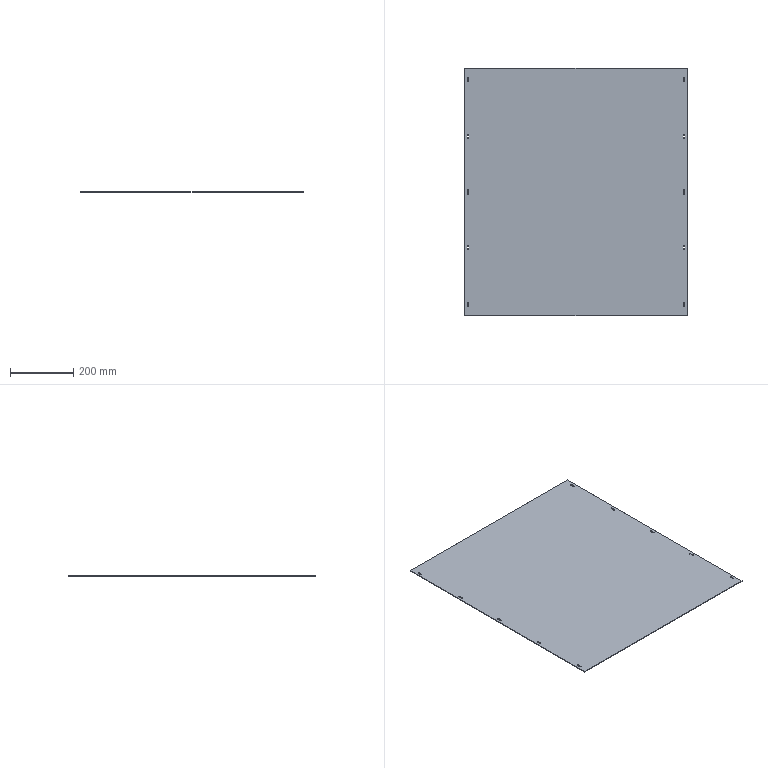Part | SolidWorks | features Extrusion 1, ICE 1 | 1 solid | 46 faces | box 700 x 780 x 2 mm | volume 1090782 mm3 | plane 26 | cylinder 20 | commonest cylinder face diameters 4.5 x20
STEP:
#1=CARTESIAN_POINT('',(350.,-390.,0.));
#2=VERTEX_POINT('',#1);
#3=CARTESIAN_POINT('',(350.,390.,0.));
#4=VERTEX_POINT('',#3);
#5=CARTESIAN_POINT('',(350.,390.,0.));
#6=DIRECTION('',(0.,1.,0.));
#7=VECTOR('',#6,1000.);
#8=LINE('',#5,#7);
#9=EDGE_CURVE('',#2,#4,#8,.T.);
#10=ORIENTED_EDGE('',*,*,#9,.T.);
#11=CARTESIAN_POINT('',(350.,390.,2.));
#12=VERTEX_POINT('',#11);
#13=CARTESIAN_POINT('',(350.,390.,2.));
#14=DIRECTION('',(0.,0.,-1.));
#15=VECTOR('',#14,1000.);
#16=LINE('',#13,#15);
#17=EDGE_CURVE('',#12,#4,#16,.T.);
#18=ORIENTED_EDGE('',*,*,#17,.F.);
#19=CARTESIAN_POINT('',(350.,-390.,2.));
#20=VERTEX_POINT('',#19);
#21=CARTESIAN_POINT('',(350.,390.,2.));
#22=DIRECTION('',(0.,1.,0.));
#23=VECTOR('',#22,1000.);
#24=LINE('',#21,#23);
#25=EDGE_CURVE('',#20,#12,#24,.T.);
#26=ORIENTED_EDGE('',*,*,#25,.F.);
#27=CARTESIAN_POINT('',(350.,-390.,2.));
#28=DIRECTION('',(0.,0.,-1.));
#29=VECTOR('',#28,1000.);
#30=LINE('',#27,#29);
#31=EDGE_CURVE('',#20,#2,#30,.T.);
#32=ORIENTED_EDGE('',*,*,#31,.T.);
#33=EDGE_LOOP('',(#10,#18,#26,#32));
#34=FACE_OUTER_BOUND('',#33,.T.);
#35=CARTESIAN_POINT('',(350.,390.,2.));
#36=DIRECTION('',(-1.,0.,0.));
#37=DIRECTION('',(0.,0.,1.));
#38=AXIS2_PLACEMENT_3D('',#35,#36,#37);
#39=PLANE('',#38);
#40=ADVANCED_FACE('',(#34),#39,.F.);
#41=CARTESIAN_POINT('',(-350.,390.,0.));
#42=VERTEX_POINT('',#41);
#43=CARTESIAN_POINT('',(-350.,390.,0.));
#44=DIRECTION('',(-1.,0.,0.));
#45=VECTOR('',#44,1000.);
#46=LINE('',#43,#45);
#47=EDGE_CURVE('',#4,#42,#46,.T.);
#48=ORIENTED_EDGE('',*,*,#47,.T.);
#49=CARTESIAN_POINT('',(-350.,390.,2.));
#50=VERTEX_POINT('',#49);
#51=CARTESIAN_POINT('',(-350.,390.,2.));
#52=DIRECTION('',(0.,0.,-1.));
#53=VECTOR('',#52,1000.);
#54=LINE('',#51,#53);
#55=EDGE_CURVE('',#50,#42,#54,.T.);
#56=ORIENTED_EDGE('',*,*,#55,.F.);
#57=CARTESIAN_POINT('',(-350.,390.,2.));
#58=DIRECTION('',(-1.,0.,0.));
#59=VECTOR('',#58,1000.);
#60=LINE('',#57,#59);
#61=EDGE_CURVE('',#12,#50,#60,.T.);
#62=ORIENTED_EDGE('',*,*,#61,.F.);
#63=ORIENTED_EDGE('',*,*,#17,.T.);
#64=EDGE_LOOP('',(#48,#56,#62,#63));
#65=FACE_OUTER_BOUND('',#64,.T.);
#66=CARTESIAN_POINT('',(-350.,390.,2.));
#67=DIRECTION('',(0.,-1.,0.));
#68=DIRECTION('',(0.,0.,-1.));
#69=AXIS2_PLACEMENT_3D('',#66,#67,#68);
#70=PLANE('',#69);
#71=ADVANCED_FACE('',(#65),#70,.F.);
#72=CARTESIAN_POINT('',(-350.,-390.,0.));
#73=VERTEX_POINT('',#72);
#74=CARTESIAN_POINT('',(-350.,390.,0.));
#75=DIRECTION('',(0.,-1.,0.));
#76=VECTOR('',#75,1000.);
#77=LINE('',#74,#76);
#78=EDGE_CURVE('',#42,#73,#77,.T.);
#79=ORIENTED_EDGE('',*,*,#78,.T.);
#80=CARTESIAN_POINT('',(-350.,-390.,2.));
#81=VERTEX_POINT('',#80);
#82=CARTESIAN_POINT('',(-350.,-390.,2.));
#83=DIRECTION('',(0.,0.,-1.));
#84=VECTOR('',#83,1000.);
#85=LINE('',#82,#84);
#86=EDGE_CURVE('',#81,#73,#85,.T.);
#87=ORIENTED_EDGE('',*,*,#86,.F.);
#88=CARTESIAN_POINT('',(-350.,390.,2.));
#89=DIRECTION('',(0.,-1.,0.));
#90=VECTOR('',#89,1000.);
#91=LINE('',#88,#90);
#92=EDGE_CURVE('',#50,#81,#91,.T.);
#93=ORIENTED_EDGE('',*,*,#92,.F.);
#94=ORIENTED_EDGE('',*,*,#55,.T.);
#95=EDGE_LOOP('',(#79,#87,#93,#94));
#96=FACE_OUTER_BOUND('',#95,.T.);
#97=CARTESIAN_POINT('',(-350.,390.,2.));
#98=DIRECTION('',(1.,0.,0.));
#99=DIRECTION('',(0.,0.,-1.));
#100=AXIS2_PLACEMENT_3D('',#97,#98,#99);
#101=PLANE('',#100);
#102=ADVANCED_FACE('',(#96),#101,.F.);
#103=CARTESIAN_POINT('',(-350.,-390.,0.));
#104=DIRECTION('',(1.,0.,0.));
#105=VECTOR('',#104,1000.);
#106=LINE('',#103,#105);
#107=EDGE_CURVE('',#73,#2,#106,.T.);
#108=ORIENTED_EDGE('',*,*,#107,.T.);
#109=ORIENTED_EDGE('',*,*,#31,.F.);
#110=CARTESIAN_POINT('',(-350.,-390.,2.));
#111=DIRECTION('',(1.,0.,0.));
#112=VECTOR('',#111,1000.);
#113=LINE('',#110,#112);
#114=EDGE_CURVE('',#81,#20,#113,.T.);
#115=ORIENTED_EDGE('',*,*,#114,.F.);
#116=ORIENTED_EDGE('',*,*,#86,.T.);
#117=EDGE_LOOP('',(#108,#109,#115,#116));
#118=FACE_OUTER_BOUND('',#117,.T.);
#119=CARTESIAN_POINT('',(-350.,-390.,2.));
#120=DIRECTION('',(0.,1.,0.));
#121=DIRECTION('',(0.,0.,1.));
#122=AXIS2_PLACEMENT_3D('',#119,#120,#121);
#123=PLANE('',#122);
#124=ADVANCED_FACE('',(#118),#123,.F.);
#125=CARTESIAN_POINT('',(337.75,-5.,2.));
#126=VERTEX_POINT('',#125);
#127=CARTESIAN_POINT('',(342.25,-5.,2.));
#128=VERTEX_POINT('',#127);
#129=CARTESIAN_POINT('',(340.,-5.,2.));
#130=DIRECTION('',(0.,0.,1.));
#131=DIRECTION('',(-1.,0.,0.));
#132=AXIS2_PLACEMENT_3D('',#129,#130,#131);
#133=CIRCLE('',#132,2.25);
#134=EDGE_CURVE('',#126,#128,#133,.T.);
#135=ORIENTED_EDGE('',*,*,#134,.F.);
#136=CARTESIAN_POINT('',(337.75,5.,2.));
#137=VERTEX_POINT('',#136);
#138=CARTESIAN_POINT('',(337.75,-5.,2.));
#139=DIRECTION('',(0.,-1.,0.));
#140=VECTOR('',#139,1000.);
#141=LINE('',#138,#140);
#142=EDGE_CURVE('',#137,#126,#141,.T.);
#143=ORIENTED_EDGE('',*,*,#142,.F.);
#144=CARTESIAN_POINT('',(342.25,5.,2.));
#145=VERTEX_POINT('',#144);
#146=CARTESIAN_POINT('',(340.,5.,2.));
#147=DIRECTION('',(0.,0.,1.));
#148=DIRECTION('',(-1.,0.,0.));
#149=AXIS2_PLACEMENT_3D('',#146,#147,#148);
#150=CIRCLE('',#149,2.25);
#151=EDGE_CURVE('',#145,#137,#150,.T.);
#152=ORIENTED_EDGE('',*,*,#151,.F.);
#153=CARTESIAN_POINT('',(342.25,-5.,2.));
#154=DIRECTION('',(0.,1.,0.));
#155=VECTOR('',#154,1000.);
#156=LINE('',#153,#155);
#157=EDGE_CURVE('',#128,#145,#156,.T.);
#158=ORIENTED_EDGE('',*,*,#157,.F.);
#159=EDGE_LOOP('',(#135,#143,#152,#158));
#160=FACE_BOUND('',#159,.T.);
#161=CARTESIAN_POINT('',(342.25,-170.,2.));
#162=VERTEX_POINT('',#161);
#163=CARTESIAN_POINT('',(337.75,-170.,2.));
#164=VERTEX_POINT('',#163);
#165=CARTESIAN_POINT('',(340.,-170.,2.));
#166=DIRECTION('',(0.,0.,1.));
#167=DIRECTION('',(1.,0.,0.));
#168=AXIS2_PLACEMENT_3D('',#165,#166,#167);
#169=CIRCLE('',#168,2.25);
#170=EDGE_CURVE('',#162,#164,#169,.T.);
#171=ORIENTED_EDGE('',*,*,#170,.F.);
#172=CARTESIAN_POINT('',(342.25,-180.,2.));
#173=VERTEX_POINT('',#172);
#174=CARTESIAN_POINT('',(342.25,-170.,2.));
#175=DIRECTION('',(0.,1.,0.));
#176=VECTOR('',#175,1000.);
#177=LINE('',#174,#176);
#178=EDGE_CURVE('',#173,#162,#177,.T.);
#179=ORIENTED_EDGE('',*,*,#178,.F.);
#180=CARTESIAN_POINT('',(337.75,-180.,2.));
#181=VERTEX_POINT('',#180);
#182=CARTESIAN_POINT('',(340.,-180.,2.));
#183=DIRECTION('',(0.,0.,1.));
#184=DIRECTION('',(1.,0.,0.));
#185=AXIS2_PLACEMENT_3D('',#182,#183,#184);
#186=CIRCLE('',#185,2.25);
#187=EDGE_CURVE('',#181,#173,#186,.T.);
#188=ORIENTED_EDGE('',*,*,#187,.F.);
#189=CARTESIAN_POINT('',(337.75,-170.,2.));
#190=DIRECTION('',(0.,-1.,0.));
#191=VECTOR('',#190,1000.);
#192=LINE('',#189,#191);
#193=EDGE_CURVE('',#164,#181,#192,.T.);
#194=ORIENTED_EDGE('',*,*,#193,.F.);
#195=EDGE_LOOP('',(#171,#179,#188,#194));
#196=FACE_BOUND('',#195,.T.);
#197=CARTESIAN_POINT('',(342.25,360.,2.));
#198=VERTEX_POINT('',#197);
#199=CARTESIAN_POINT('',(337.75,360.,2.));
#200=VERTEX_POINT('',#199);
#201=CARTESIAN_POINT('',(340.,360.,2.));
#202=DIRECTION('',(0.,0.,1.));
#203=DIRECTION('',(-1.,0.,0.));
#204=AXIS2_PLACEMENT_3D('',#201,#202,#203);
#205=CIRCLE('',#204,2.25);
#206=EDGE_CURVE('',#198,#200,#205,.T.);
#207=ORIENTED_EDGE('',*,*,#206,.F.);
#208=CARTESIAN_POINT('',(342.25,350.,2.));
#209=VERTEX_POINT('',#208);
#210=CARTESIAN_POINT('',(342.25,360.,2.));
#211=DIRECTION('',(0.,1.,0.));
#212=VECTOR('',#211,1000.);
#213=LINE('',#210,#212);
#214=EDGE_CURVE('',#209,#198,#213,.T.);
#215=ORIENTED_EDGE('',*,*,#214,.F.);
#216=CARTESIAN_POINT('',(337.75,350.,2.));
#217=VERTEX_POINT('',#216);
#218=CARTESIAN_POINT('',(340.,350.,2.));
#219=DIRECTION('',(0.,0.,1.));
#220=DIRECTION('',(-1.,0.,0.));
#221=AXIS2_PLACEMENT_3D('',#218,#219,#220);
#222=CIRCLE('',#221,2.25);
#223=EDGE_CURVE('',#217,#209,#222,.T.);
#224=ORIENTED_EDGE('',*,*,#223,.F.);
#225=CARTESIAN_POINT('',(337.75,360.,2.));
#226=DIRECTION('',(0.,-1.,0.));
#227=VECTOR('',#226,1000.);
#228=LINE('',#225,#227);
#229=EDGE_CURVE('',#200,#217,#228,.T.);
#230=ORIENTED_EDGE('',*,*,#229,.F.);
#231=EDGE_LOOP('',(#207,#215,#224,#230));
#232=FACE_BOUND('',#231,.T.);
#233=CARTESIAN_POINT('',(-342.25,170.,2.));
#234=VERTEX_POINT('',#233);
#235=CARTESIAN_POINT('',(-337.75,170.,2.));
#236=VERTEX_POINT('',#235);
#237=CARTESIAN_POINT('',(-340.,170.,2.));
#238=DIRECTION('',(0.,0.,1.));
#239=DIRECTION('',(1.,0.,0.));
#240=AXIS2_PLACEMENT_3D('',#237,#238,#239);
#241=CIRCLE('',#240,2.25);
#242=EDGE_CURVE('',#234,#236,#241,.T.);
#243=ORIENTED_EDGE('',*,*,#242,.F.);
#244=CARTESIAN_POINT('',(-342.25,180.,2.));
#245=VERTEX_POINT('',#244);
#246=CARTESIAN_POINT('',(-342.25,170.,2.));
#247=DIRECTION('',(0.,-1.,0.));
#248=VECTOR('',#247,1000.);
#249=LINE('',#246,#248);
#250=EDGE_CURVE('',#245,#234,#249,.T.);
#251=ORIENTED_EDGE('',*,*,#250,.F.);
#252=CARTESIAN_POINT('',(-337.75,180.,2.));
#253=VERTEX_POINT('',#252);
#254=CARTESIAN_POINT('',(-340.,180.,2.));
#255=DIRECTION('',(0.,0.,1.));
#256=DIRECTION('',(1.,0.,0.));
#257=AXIS2_PLACEMENT_3D('',#254,#255,#256);
#258=CIRCLE('',#257,2.25);
#259=EDGE_CURVE('',#253,#245,#258,.T.);
#260=ORIENTED_EDGE('',*,*,#259,.F.);
#261=CARTESIAN_POINT('',(-337.75,170.,2.));
#262=DIRECTION('',(0.,1.,0.));
#263=VECTOR('',#262,1000.);
#264=LINE('',#261,#263);
#265=EDGE_CURVE('',#236,#253,#264,.T.);
#266=ORIENTED_EDGE('',*,*,#265,.F.);
#267=EDGE_LOOP('',(#243,#251,#260,#266));
#268=FACE_BOUND('',#267,.T.);
#269=CARTESIAN_POINT('',(-342.25,-5.,2.));
#270=VERTEX_POINT('',#269);
#271=CARTESIAN_POINT('',(-337.75,-5.,2.));
#272=VERTEX_POINT('',#271);
#273=CARTESIAN_POINT('',(-340.,-5.,2.));
#274=DIRECTION('',(0.,0.,1.));
#275=DIRECTION('',(1.,0.,0.));
#276=AXIS2_PLACEMENT_3D('',#273,#274,#275);
#277=CIRCLE('',#276,2.25);
#278=EDGE_CURVE('',#270,#272,#277,.T.);
#279=ORIENTED_EDGE('',*,*,#278,.F.);
#280=CARTESIAN_POINT('',(-342.25,5.,2.));
#281=VERTEX_POINT('',#280);
#282=CARTESIAN_POINT('',(-342.25,-5.,2.));
#283=DIRECTION('',(0.,-1.,0.));
#284=VECTOR('',#283,1000.);
#285=LINE('',#282,#284);
#286=EDGE_CURVE('',#281,#270,#285,.T.);
#287=ORIENTED_EDGE('',*,*,#286,.F.);
#288=CARTESIAN_POINT('',(-337.75,5.,2.));
#289=VERTEX_POINT('',#288);
#290=CARTESIAN_POINT('',(-340.,5.,2.));
#291=DIRECTION('',(0.,0.,1.));
#292=DIRECTION('',(1.,0.,0.));
#293=AXIS2_PLACEMENT_3D('',#290,#291,#292);
#294=CIRCLE('',#293,2.25);
#295=EDGE_CURVE('',#289,#281,#294,.T.);
#296=ORIENTED_EDGE('',*,*,#295,.F.);
#297=CARTESIAN_POINT('',(-337.75,-5.,2.));
#298=DIRECTION('',(0.,1.,0.));
#299=VECTOR('',#298,1000.);
#300=LINE('',#297,#299);
#301=EDGE_CURVE('',#272,#289,#300,.T.);
#302=ORIENTED_EDGE('',*,*,#301,.F.);
#303=EDGE_LOOP('',(#279,#287,#296,#302));
#304=FACE_BOUND('',#303,.T.);
#305=CARTESIAN_POINT('',(337.75,170.,2.));
#306=VERTEX_POINT('',#305);
#307=CARTESIAN_POINT('',(342.25,170.,2.));
#308=VERTEX_POINT('',#307);
#309=CARTESIAN_POINT('',(340.,170.,2.));
#310=DIRECTION('',(0.,0.,1.));
#311=DIRECTION('',(-1.,0.,0.));
#312=AXIS2_PLACEMENT_3D('',#309,#310,#311);
#313=CIRCLE('',#312,2.25);
#314=EDGE_CURVE('',#306,#308,#313,.T.);
#315=ORIENTED_EDGE('',*,*,#314,.F.);
#316=CARTESIAN_POINT('',(337.75,180.,2.));
#317=VERTEX_POINT('',#316);
#318=CARTESIAN_POINT('',(337.75,170.,2.));
#319=DIRECTION('',(0.,-1.,0.));
#320=VECTOR('',#319,1000.);
#321=LINE('',#318,#320);
#322=EDGE_CURVE('',#317,#306,#321,.T.);
#323=ORIENTED_EDGE('',*,*,#322,.F.);
#324=CARTESIAN_POINT('',(342.25,180.,2.));
#325=VERTEX_POINT('',#324);
#326=CARTESIAN_POINT('',(340.,180.,2.));
#327=DIRECTION('',(0.,0.,1.));
#328=DIRECTION('',(-1.,0.,0.));
#329=AXIS2_PLACEMENT_3D('',#326,#327,#328);
#330=CIRCLE('',#329,2.25);
#331=EDGE_CURVE('',#325,#317,#330,.T.);
#332=ORIENTED_EDGE('',*,*,#331,.F.);
#333=CARTESIAN_POINT('',(342.25,170.,2.));
#334=DIRECTION('',(0.,1.,0.));
#335=VECTOR('',#334,1000.);
#336=LINE('',#333,#335);
#337=EDGE_CURVE('',#308,#325,#336,.T.);
#338=ORIENTED_EDGE('',*,*,#337,.F.);
#339=EDGE_LOOP('',(#315,#323,#332,#338));
#340=FACE_BOUND('',#339,.T.);
#341=CARTESIAN_POINT('',(-342.25,-360.,2.));
#342=VERTEX_POINT('',#341);
#343=CARTESIAN_POINT('',(-337.75,-360.,2.));
#344=VERTEX_POINT('',#343);
#345=CARTESIAN_POINT('',(-340.,-360.,2.));
#346=DIRECTION('',(0.,0.,1.));
#347=DIRECTION('',(-1.,0.,0.));
#348=AXIS2_PLACEMENT_3D('',#345,#346,#347);
#349=CIRCLE('',#348,2.25);
#350=EDGE_CURVE('',#342,#344,#349,.T.);
#351=ORIENTED_EDGE('',*,*,#350,.F.);
#352=CARTESIAN_POINT('',(-342.25,-350.,2.));
#353=VERTEX_POINT('',#352);
#354=CARTESIAN_POINT('',(-342.25,-360.,2.));
#355=DIRECTION('',(0.,-1.,0.));
#356=VECTOR('',#355,1000.);
#357=LINE('',#354,#356);
#358=EDGE_CURVE('',#353,#342,#357,.T.);
#359=ORIENTED_EDGE('',*,*,#358,.F.);
#360=CARTESIAN_POINT('',(-337.75,-350.,2.));
#361=VERTEX_POINT('',#360);
#362=CARTESIAN_POINT('',(-340.,-350.,2.));
#363=DIRECTION('',(0.,0.,1.));
#364=DIRECTION('',(-1.,0.,0.));
#365=AXIS2_PLACEMENT_3D('',#362,#363,#364);
#366=CIRCLE('',#365,2.25);
#367=EDGE_CURVE('',#361,#353,#366,.T.);
#368=ORIENTED_EDGE('',*,*,#367,.F.);
#369=CARTESIAN_POINT('',(-337.75,-360.,2.));
#370=DIRECTION('',(0.,1.,0.));
#371=VECTOR('',#370,1000.);
#372=LINE('',#369,#371);
#373=EDGE_CURVE('',#344,#361,#372,.T.);
#374=ORIENTED_EDGE('',*,*,#373,.F.);
#375=EDGE_LOOP('',(#351,#359,#368,#374));
#376=FACE_BOUND('',#375,.T.);
#377=CARTESIAN_POINT('',(337.75,-360.,2.));
#378=VERTEX_POINT('',#377);
#379=CARTESIAN_POINT('',(342.25,-360.,2.));
#380=VERTEX_POINT('',#379);
#381=CARTESIAN_POINT('',(340.,-360.,2.));
#382=DIRECTION('',(0.,0.,1.));
#383=DIRECTION('',(1.,0.,0.));
#384=AXIS2_PLACEMENT_3D('',#381,#382,#383);
#385=CIRCLE('',#384,2.25);
#386=EDGE_CURVE('',#378,#380,#385,.T.);
#387=ORIENTED_EDGE('',*,*,#386,.F.);
#388=CARTESIAN_POINT('',(337.75,-350.,2.));
#389=VERTEX_POINT('',#388);
#390=CARTESIAN_POINT('',(337.75,-360.,2.));
#391=DIRECTION('',(0.,-1.,0.));
#392=VECTOR('',#391,1000.);
#393=LINE('',#390,#392);
#394=EDGE_CURVE('',#389,#378,#393,.T.);
#395=ORIENTED_EDGE('',*,*,#394,.F.);
#396=CARTESIAN_POINT('',(342.25,-350.,2.));
#397=VERTEX_POINT('',#396);
#398=CARTESIAN_POINT('',(340.,-350.,2.));
#399=DIRECTION('',(0.,0.,1.));
#400=DIRECTION('',(1.,0.,0.));
#401=AXIS2_PLACEMENT_3D('',#398,#399,#400);
#402=CIRCLE('',#401,2.25);
#403=EDGE_CURVE('',#397,#389,#402,.T.);
#404=ORIENTED_EDGE('',*,*,#403,.F.);
#405=CARTESIAN_POINT('',(342.25,-360.,2.));
#406=DIRECTION('',(0.,1.,0.));
#407=VECTOR('',#406,1000.);
#408=LINE('',#405,#407);
#409=EDGE_CURVE('',#380,#397,#408,.T.);
#410=ORIENTED_EDGE('',*,*,#409,.F.);
#411=EDGE_LOOP('',(#387,#395,#404,#410));
#412=FACE_BOUND('',#411,.T.);
#413=CARTESIAN_POINT('',(-337.75,-170.,2.));
#414=VERTEX_POINT('',#413);
#415=CARTESIAN_POINT('',(-342.25,-170.,2.));
#416=VERTEX_POINT('',#415);
#417=CARTESIAN_POINT('',(-340.,-170.,2.));
#418=DIRECTION('',(0.,0.,1.));
#419=DIRECTION('',(-1.,0.,0.));
#420=AXIS2_PLACEMENT_3D('',#417,#418,#419);
#421=CIRCLE('',#420,2.25);
#422=EDGE_CURVE('',#414,#416,#421,.T.);
#423=ORIENTED_EDGE('',*,*,#422,.F.);
#424=CARTESIAN_POINT('',(-337.75,-180.,2.));
#425=VERTEX_POINT('',#424);
#426=CARTESIAN_POINT('',(-337.75,-170.,2.));
#427=DIRECTION('',(0.,1.,0.));
#428=VECTOR('',#427,1000.);
#429=LINE('',#426,#428);
#430=EDGE_CURVE('',#425,#414,#429,.T.);
#431=ORIENTED_EDGE('',*,*,#430,.F.);
#432=CARTESIAN_POINT('',(-342.25,-180.,2.));
#433=VERTEX_POINT('',#432);
#434=CARTESIAN_POINT('',(-340.,-180.,2.));
#435=DIRECTION('',(0.,0.,1.));
#436=DIRECTION('',(-1.,0.,0.));
#437=AXIS2_PLACEMENT_3D('',#434,#435,#436);
#438=CIRCLE('',#437,2.25);
#439=EDGE_CURVE('',#433,#425,#438,.T.);
#440=ORIENTED_EDGE('',*,*,#439,.F.);
#441=CARTESIAN_POINT('',(-342.25,-170.,2.));
#442=DIRECTION('',(0.,-1.,0.));
#443=VECTOR('',#442,1000.);
#444=LINE('',#441,#443);
#445=EDGE_CURVE('',#416,#433,#444,.T.);
#446=ORIENTED_EDGE('',*,*,#445,.F.);
#447=EDGE_LOOP('',(#423,#431,#440,#446));
#448=FACE_BOUND('',#447,.T.);
#449=CARTESIAN_POINT('',(-337.75,360.,2.));
#450=VERTEX_POINT('',#449);
#451=CARTESIAN_POINT('',(-342.25,360.,2.));
#452=VERTEX_POINT('',#451);
#453=CARTESIAN_POINT('',(-340.,360.,2.));
#454=DIRECTION('',(0.,0.,1.));
#455=DIRECTION('',(1.,0.,0.));
#456=AXIS2_PLACEMENT_3D('',#453,#454,#455);
#457=CIRCLE('',#456,2.25);
#458=EDGE_CURVE('',#450,#452,#457,.T.);
#459=ORIENTED_EDGE('',*,*,#458,.F.);
#460=CARTESIAN_POINT('',(-337.75,350.,2.));
#461=VERTEX_POINT('',#460);
#462=CARTESIAN_POINT('',(-337.75,360.,2.));
#463=DIRECTION('',(0.,1.,0.));
#464=VECTOR('',#463,1000.);
#465=LINE('',#462,#464);
#466=EDGE_CURVE('',#461,#450,#465,.T.);
#467=ORIENTED_EDGE('',*,*,#466,.F.);
#468=CARTESIAN_POINT('',(-342.25,350.,2.));
#469=VERTEX_POINT('',#468);
#470=CARTESIAN_POINT('',(-340.,350.,2.));
#471=DIRECTION('',(0.,0.,1.));
#472=DIRECTION('',(1.,0.,0.));
#473=AXIS2_PLACEMENT_3D('',#470,#471,#472);
#474=CIRCLE('',#473,2.25);
#475=EDGE_CURVE('',#469,#461,#474,.T.);
#476=ORIENTED_EDGE('',*,*,#475,.F.);
#477=CARTESIAN_POINT('',(-342.25,360.,2.));
#478=DIRECTION('',(0.,-1.,0.));
#479=VECTOR('',#478,1000.);
#480=LINE('',#477,#479);
#481=EDGE_CURVE('',#452,#469,#480,.T.);
#482=ORIENTED_EDGE('',*,*,#481,.F.);
#483=EDGE_LOOP('',(#459,#467,#476,#482));
#484=FACE_BOUND('',#483,.T.);
#485=ORIENTED_EDGE('',*,*,#25,.T.);
#486=ORIENTED_EDGE('',*,*,#61,.T.);
#487=ORIENTED_EDGE('',*,*,#92,.T.);
#488=ORIENTED_EDGE('',*,*,#114,.T.);
#489=EDGE_LOOP('',(#485,#486,#487,#488));
#490=FACE_OUTER_BOUND('',#489,.T.);
#491=CARTESIAN_POINT('',(0.,0.,2.));
#492=DIRECTION('',(0.,0.,1.));
#493=DIRECTION('',(1.,0.,0.));
#494=AXIS2_PLACEMENT_3D('',#491,#492,#493);
#495=PLANE('',#494);
#496=ADVANCED_FACE('',(#160,#196,#232,#268,#304,#340,#376,#412,#448,#484,#490),#495,.T.);
#497=CARTESIAN_POINT('',(337.75,5.,0.));
#498=VERTEX_POINT('',#497);
#499=CARTESIAN_POINT('',(337.75,-5.,0.));
#500=VERTEX_POINT('',#499);
#501=CARTESIAN_POINT('',(337.75,0.,0.));
#502=DIRECTION('',(0.,-1.,0.));
#503=VECTOR('',#502,1000.);
#504=LINE('',#501,#503);
#505=EDGE_CURVE('',#498,#500,#504,.T.);
#506=ORIENTED_EDGE('',*,*,#505,.T.);
#507=CARTESIAN_POINT('',(342.25,-5.,0.));
#508=VERTEX_POINT('',#507);
#509=CARTESIAN_POINT('',(340.,-5.,0.));
#510=DIRECTION('',(0.,0.,1.));
#511=DIRECTION('',(1.,0.,0.));
#512=AXIS2_PLACEMENT_3D('',#509,#510,#511);
#513=CIRCLE('',#512,2.25);
#514=EDGE_CURVE('',#500,#508,#513,.T.);
#515=ORIENTED_EDGE('',*,*,#514,.T.);
#516=CARTESIAN_POINT('',(342.25,5.,0.));
#517=VERTEX_POINT('',#516);
#518=CARTESIAN_POINT('',(342.25,0.,0.));
#519=DIRECTION('',(0.,1.,0.));
#520=VECTOR('',#519,1000.);
#521=LINE('',#518,#520);
#522=EDGE_CURVE('',#508,#517,#521,.T.);
#523=ORIENTED_EDGE('',*,*,#522,.T.);
#524=CARTESIAN_POINT('',(340.,5.,0.));
#525=DIRECTION('',(0.,0.,1.));
#526=DIRECTION('',(1.,0.,0.));
#527=AXIS2_PLACEMENT_3D('',#524,#525,#526);
#528=CIRCLE('',#527,2.25);
#529=EDGE_CURVE('',#517,#498,#528,.T.);
#530=ORIENTED_EDGE('',*,*,#529,.T.);
#531=EDGE_LOOP('',(#506,#515,#523,#530));
#532=FACE_BOUND('',#531,.T.);
#533=CARTESIAN_POINT('',(342.25,-180.,0.));
#534=VERTEX_POINT('',#533);
#535=CARTESIAN_POINT('',(342.25,-170.,0.));
#536=VERTEX_POINT('',#535);
#537=CARTESIAN_POINT('',(342.25,0.,0.));
#538=DIRECTION('',(0.,1.,0.));
#539=VECTOR('',#538,1000.);
#540=LINE('',#537,#539);
#541=EDGE_CURVE('',#534,#536,#540,.T.);
#542=ORIENTED_EDGE('',*,*,#541,.T.);
#543=CARTESIAN_POINT('',(337.75,-170.,0.));
#544=VERTEX_POINT('',#543);
#545=CARTESIAN_POINT('',(340.,-170.,0.));
#546=DIRECTION('',(0.,0.,1.));
#547=DIRECTION('',(1.,0.,0.));
#548=AXIS2_PLACEMENT_3D('',#545,#546,#547);
#549=CIRCLE('',#548,2.25);
#550=EDGE_CURVE('',#536,#544,#549,.T.);
#551=ORIENTED_EDGE('',*,*,#550,.T.);
#552=CARTESIAN_POINT('',(337.75,-180.,0.));
#553=VERTEX_POINT('',#552);
#554=CARTESIAN_POINT('',(337.75,0.,0.));
#555=DIRECTION('',(0.,-1.,0.));
#556=VECTOR('',#555,1000.);
#557=LINE('',#554,#556);
#558=EDGE_CURVE('',#544,#553,#557,.T.);
#559=ORIENTED_EDGE('',*,*,#558,.T.);
#560=CARTESIAN_POINT('',(340.,-180.,0.));
#561=DIRECTION('',(0.,0.,1.));
#562=DIRECTION('',(1.,0.,0.));
#563=AXIS2_PLACEMENT_3D('',#560,#561,#562);
#564=CIRCLE('',#563,2.25);
#565=EDGE_CURVE('',#553,#534,#564,.T.);
#566=ORIENTED_EDGE('',*,*,#565,.T.);
#567=EDGE_LOOP('',(#542,#551,#559,#566));
#568=FACE_BOUND('',#567,.T.);
#569=CARTESIAN_POINT('',(342.25,350.,0.));
#570=VERTEX_POINT('',#569);
#571=CARTESIAN_POINT('',(342.25,360.,0.));
#572=VERTEX_POINT('',#571);
#573=CARTESIAN_POINT('',(342.25,0.,0.));
#574=DIRECTION('',(0.,1.,0.));
#575=VECTOR('',#574,1000.);
#576=LINE('',#573,#575);
#577=EDGE_CURVE('',#570,#572,#576,.T.);
#578=ORIENTED_EDGE('',*,*,#577,.T.);
#579=CARTESIAN_POINT('',(337.75,360.,0.));
#580=VERTEX_POINT('',#579);
#581=CARTESIAN_POINT('',(340.,360.,0.));
#582=DIRECTION('',(0.,0.,1.));
#583=DIRECTION('',(1.,0.,0.));
#584=AXIS2_PLACEMENT_3D('',#581,#582,#583);
#585=CIRCLE('',#584,2.25);
#586=EDGE_CURVE('',#572,#580,#585,.T.);
#587=ORIENTED_EDGE('',*,*,#586,.T.);
#588=CARTESIAN_POINT('',(337.75,350.,0.));
#589=VERTEX_POINT('',#588);
#590=CARTESIAN_POINT('',(337.75,0.,0.));
#591=DIRECTION('',(0.,-1.,0.));
#592=VECTOR('',#591,1000.);
#593=LINE('',#590,#592);
#594=EDGE_CURVE('',#580,#589,#593,.T.);
#595=ORIENTED_EDGE('',*,*,#594,.T.);
#596=CARTESIAN_POINT('',(340.,350.,0.));
#597=DIRECTION('',(0.,0.,1.));
#598=DIRECTION('',(1.,0.,0.));
#599=AXIS2_PLACEMENT_3D('',#596,#597,#598);
#600=CIRCLE('',#599,2.25);
#601=EDGE_CURVE('',#589,#570,#600,.T.);
#602=ORIENTED_EDGE('',*,*,#601,.T.);
#603=EDGE_LOOP('',(#578,#587,#595,#602));
#604=FACE_BOUND('',#603,.T.);
#605=CARTESIAN_POINT('',(-342.25,180.,0.));
#606=VERTEX_POINT('',#605);
#607=CARTESIAN_POINT('',(-342.25,170.,0.));
#608=VERTEX_POINT('',#607);
#609=CARTESIAN_POINT('',(-342.25,0.,0.));
#610=DIRECTION('',(0.,-1.,0.));
#611=VECTOR('',#610,1000.);
#612=LINE('',#609,#611);
#613=EDGE_CURVE('',#606,#608,#612,.T.);
#614=ORIENTED_EDGE('',*,*,#613,.T.);
#615=CARTESIAN_POINT('',(-337.75,170.,0.));
#616=VERTEX_POINT('',#615);
#617=CARTESIAN_POINT('',(-340.,170.,0.));
#618=DIRECTION('',(0.,0.,1.));
#619=DIRECTION('',(1.,0.,0.));
#620=AXIS2_PLACEMENT_3D('',#617,#618,#619);
#621=CIRCLE('',#620,2.25);
#622=EDGE_CURVE('',#608,#616,#621,.T.);
#623=ORIENTED_EDGE('',*,*,#622,.T.);
#624=CARTESIAN_POINT('',(-337.75,180.,0.));
#625=VERTEX_POINT('',#624);
#626=CARTESIAN_POINT('',(-337.75,0.,0.));
#627=DIRECTION('',(0.,1.,0.));
#628=VECTOR('',#627,1000.);
#629=LINE('',#626,#628);
#630=EDGE_CURVE('',#616,#625,#629,.T.);
#631=ORIENTED_EDGE('',*,*,#630,.T.);
#632=CARTESIAN_POINT('',(-340.,180.,0.));
#633=DIRECTION('',(0.,0.,1.));
#634=DIRECTION('',(1.,0.,0.));
#635=AXIS2_PLACEMENT_3D('',#632,#633,#634);
#636=CIRCLE('',#635,2.25);
#637=EDGE_CURVE('',#625,#606,#636,.T.);
#638=ORIENTED_EDGE('',*,*,#637,.T.);
#639=EDGE_LOOP('',(#614,#623,#631,#638));
#640=FACE_BOUND('',#639,.T.);
#641=CARTESIAN_POINT('',(-342.25,5.,0.));
#642=VERTEX_POINT('',#641);
#643=CARTESIAN_POINT('',(-342.25,-5.,0.));
#644=VERTEX_POINT('',#643);
#645=CARTESIAN_POINT('',(-342.25,0.,0.));
#646=DIRECTION('',(0.,-1.,0.));
#647=VECTOR('',#646,1000.);
#648=LINE('',#645,#647);
#649=EDGE_CURVE('',#642,#644,#648,.T.);
#650=ORIENTED_EDGE('',*,*,#649,.T.);
#651=CARTESIAN_POINT('',(-337.75,-5.,0.));
#652=VERTEX_POINT('',#651);
#653=CARTESIAN_POINT('',(-340.,-5.,0.));
#654=DIRECTION('',(0.,0.,1.));
#655=DIRECTION('',(1.,0.,0.));
#656=AXIS2_PLACEMENT_3D('',#653,#654,#655);
#657=CIRCLE('',#656,2.25);
#658=EDGE_CURVE('',#644,#652,#657,.T.);
#659=ORIENTED_EDGE('',*,*,#658,.T.);
#660=CARTESIAN_POINT('',(-337.75,5.,0.));
#661=VERTEX_POINT('',#660);
#662=CARTESIAN_POINT('',(-337.75,0.,0.));
#663=DIRECTION('',(0.,1.,0.));
#664=VECTOR('',#663,1000.);
#665=LINE('',#662,#664);
#666=EDGE_CURVE('',#652,#661,#665,.T.);
#667=ORIENTED_EDGE('',*,*,#666,.T.);
#668=CARTESIAN_POINT('',(-340.,5.,0.));
#669=DIRECTION('',(0.,0.,1.));
#670=DIRECTION('',(1.,0.,0.));
#671=AXIS2_PLACEMENT_3D('',#668,#669,#670);
#672=CIRCLE('',#671,2.25);
#673=EDGE_CURVE('',#661,#642,#672,.T.);
#674=ORIENTED_EDGE('',*,*,#673,.T.);
#675=EDGE_LOOP('',(#650,#659,#667,#674));
#676=FACE_BOUND('',#675,.T.);
#677=CARTESIAN_POINT('',(337.75,180.,0.));
#678=VERTEX_POINT('',#677);
#679=CARTESIAN_POINT('',(337.75,170.,0.));
#680=VERTEX_POINT('',#679);
#681=CARTESIAN_POINT('',(337.75,0.,0.));
#682=DIRECTION('',(0.,-1.,0.));
#683=VECTOR('',#682,1000.);
#684=LINE('',#681,#683);
#685=EDGE_CURVE('',#678,#680,#684,.T.);
#686=ORIENTED_EDGE('',*,*,#685,.T.);
#687=CARTESIAN_POINT('',(342.25,170.,0.));
#688=VERTEX_POINT('',#687);
#689=CARTESIAN_POINT('',(340.,170.,0.));
#690=DIRECTION('',(0.,0.,1.));
#691=DIRECTION('',(1.,0.,0.));
#692=AXIS2_PLACEMENT_3D('',#689,#690,#691);
#693=CIRCLE('',#692,2.25);
#694=EDGE_CURVE('',#680,#688,#693,.T.);
#695=ORIENTED_EDGE('',*,*,#694,.T.);
#696=CARTESIAN_POINT('',(342.25,180.,0.));
#697=VERTEX_POINT('',#696);
#698=CARTESIAN_POINT('',(342.25,0.,0.));
#699=DIRECTION('',(0.,1.,0.));
#700=VECTOR('',#699,1000.);
#701=LINE('',#698,#700);
#702=EDGE_CURVE('',#688,#697,#701,.T.);
#703=ORIENTED_EDGE('',*,*,#702,.T.);
#704=CARTESIAN_POINT('',(340.,180.,0.));
#705=DIRECTION('',(0.,0.,1.));
#706=DIRECTION('',(1.,0.,0.));
#707=AXIS2_PLACEMENT_3D('',#704,#705,#706);
#708=CIRCLE('',#707,2.25);
#709=EDGE_CURVE('',#697,#678,#708,.T.);
#710=ORIENTED_EDGE('',*,*,#709,.T.);
#711=EDGE_LOOP('',(#686,#695,#703,#710));
#712=FACE_BOUND('',#711,.T.);
#713=CARTESIAN_POINT('',(-342.25,-350.,0.));
#714=VERTEX_POINT('',#713);
#715=CARTESIAN_POINT('',(-342.25,-360.,0.));
#716=VERTEX_POINT('',#715);
#717=CARTESIAN_POINT('',(-342.25,0.,0.));
#718=DIRECTION('',(0.,-1.,0.));
#719=VECTOR('',#718,1000.);
#720=LINE('',#717,#719);
#721=EDGE_CURVE('',#714,#716,#720,.T.);
#722=ORIENTED_EDGE('',*,*,#721,.T.);
#723=CARTESIAN_POINT('',(-337.75,-360.,0.));
#724=VERTEX_POINT('',#723);
#725=CARTESIAN_POINT('',(-340.,-360.,0.));
#726=DIRECTION('',(0.,0.,1.));
#727=DIRECTION('',(1.,0.,0.));
#728=AXIS2_PLACEMENT_3D('',#725,#726,#727);
#729=CIRCLE('',#728,2.25);
#730=EDGE_CURVE('',#716,#724,#729,.T.);
#731=ORIENTED_EDGE('',*,*,#730,.T.);
#732=CARTESIAN_POINT('',(-337.75,-350.,0.));
#733=VERTEX_POINT('',#732);
#734=CARTESIAN_POINT('',(-337.75,0.,0.));
#735=DIRECTION('',(0.,1.,0.));
#736=VECTOR('',#735,1000.);
#737=LINE('',#734,#736);
#738=EDGE_CURVE('',#724,#733,#737,.T.);
#739=ORIENTED_EDGE('',*,*,#738,.T.);
#740=CARTESIAN_POINT('',(-340.,-350.,0.));
#741=DIRECTION('',(0.,0.,1.));
#742=DIRECTION('',(1.,0.,0.));
#743=AXIS2_PLACEMENT_3D('',#740,#741,#742);
#744=CIRCLE('',#743,2.25);
#745=EDGE_CURVE('',#733,#714,#744,.T.);
#746=ORIENTED_EDGE('',*,*,#745,.T.);
#747=EDGE_LOOP('',(#722,#731,#739,#746));
#748=FACE_BOUND('',#747,.T.);
#749=CARTESIAN_POINT('',(337.75,-350.,0.));
#750=VERTEX_POINT('',#749);
#751=CARTESIAN_POINT('',(337.75,-360.,0.));
#752=VERTEX_POINT('',#751);
#753=CARTESIAN_POINT('',(337.75,0.,0.));
#754=DIRECTION('',(0.,-1.,0.));
#755=VECTOR('',#754,1000.);
#756=LINE('',#753,#755);
#757=EDGE_CURVE('',#750,#752,#756,.T.);
#758=ORIENTED_EDGE('',*,*,#757,.T.);
#759=CARTESIAN_POINT('',(342.25,-360.,0.));
#760=VERTEX_POINT('',#759);
#761=CARTESIAN_POINT('',(340.,-360.,0.));
#762=DIRECTION('',(0.,0.,1.));
#763=DIRECTION('',(1.,0.,0.));
#764=AXIS2_PLACEMENT_3D('',#761,#762,#763);
#765=CIRCLE('',#764,2.25);
#766=EDGE_CURVE('',#752,#760,#765,.T.);
#767=ORIENTED_EDGE('',*,*,#766,.T.);
#768=CARTESIAN_POINT('',(342.25,-350.,0.));
#769=VERTEX_POINT('',#768);
#770=CARTESIAN_POINT('',(342.25,0.,0.));
#771=DIRECTION('',(0.,1.,0.));
#772=VECTOR('',#771,1000.);
#773=LINE('',#770,#772);
#774=EDGE_CURVE('',#760,#769,#773,.T.);
#775=ORIENTED_EDGE('',*,*,#774,.T.);
#776=CARTESIAN_POINT('',(340.,-350.,0.));
#777=DIRECTION('',(0.,0.,1.));
#778=DIRECTION('',(1.,0.,0.));
#779=AXIS2_PLACEMENT_3D('',#776,#777,#778);
#780=CIRCLE('',#779,2.25);
#781=EDGE_CURVE('',#769,#750,#780,.T.);
#782=ORIENTED_EDGE('',*,*,#781,.T.);
#783=EDGE_LOOP('',(#758,#767,#775,#782));
#784=FACE_BOUND('',#783,.T.);
#785=CARTESIAN_POINT('',(-337.75,-180.,0.));
#786=VERTEX_POINT('',#785);
#787=CARTESIAN_POINT('',(-337.75,-170.,0.));
#788=VERTEX_POINT('',#787);
#789=CARTESIAN_POINT('',(-337.75,0.,0.));
#790=DIRECTION('',(0.,1.,0.));
#791=VECTOR('',#790,1000.);
#792=LINE('',#789,#791);
#793=EDGE_CURVE('',#786,#788,#792,.T.);
#794=ORIENTED_EDGE('',*,*,#793,.T.);
#795=CARTESIAN_POINT('',(-342.25,-170.,0.));
#796=VERTEX_POINT('',#795);
#797=CARTESIAN_POINT('',(-340.,-170.,0.));
#798=DIRECTION('',(0.,0.,1.));
#799=DIRECTION('',(1.,0.,0.));
#800=AXIS2_PLACEMENT_3D('',#797,#798,#799);
#801=CIRCLE('',#800,2.25);
#802=EDGE_CURVE('',#788,#796,#801,.T.);
#803=ORIENTED_EDGE('',*,*,#802,.T.);
#804=CARTESIAN_POINT('',(-342.25,-180.,0.));
#805=VERTEX_POINT('',#804);
#806=CARTESIAN_POINT('',(-342.25,0.,0.));
#807=DIRECTION('',(0.,-1.,0.));
#808=VECTOR('',#807,1000.);
#809=LINE('',#806,#808);
#810=EDGE_CURVE('',#796,#805,#809,.T.);
#811=ORIENTED_EDGE('',*,*,#810,.T.);
#812=CARTESIAN_POINT('',(-340.,-180.,0.));
#813=DIRECTION('',(0.,0.,1.));
#814=DIRECTION('',(1.,0.,0.));
#815=AXIS2_PLACEMENT_3D('',#812,#813,#814);
#816=CIRCLE('',#815,2.25);
#817=EDGE_CURVE('',#805,#786,#816,.T.);
#818=ORIENTED_EDGE('',*,*,#817,.T.);
#819=EDGE_LOOP('',(#794,#803,#811,#818));
#820=FACE_BOUND('',#819,.T.);
#821=CARTESIAN_POINT('',(-337.75,350.,0.));
#822=VERTEX_POINT('',#821);
#823=CARTESIAN_POINT('',(-337.75,360.,0.));
#824=VERTEX_POINT('',#823);
#825=CARTESIAN_POINT('',(-337.75,0.,0.));
#826=DIRECTION('',(0.,1.,0.));
#827=VECTOR('',#826,1000.);
#828=LINE('',#825,#827);
#829=EDGE_CURVE('',#822,#824,#828,.T.);
#830=ORIENTED_EDGE('',*,*,#829,.T.);
#831=CARTESIAN_POINT('',(-342.25,360.,0.));
#832=VERTEX_POINT('',#831);
#833=CARTESIAN_POINT('',(-340.,360.,0.));
#834=DIRECTION('',(0.,0.,1.));
#835=DIRECTION('',(1.,0.,0.));
#836=AXIS2_PLACEMENT_3D('',#833,#834,#835);
#837=CIRCLE('',#836,2.25);
#838=EDGE_CURVE('',#824,#832,#837,.T.);
#839=ORIENTED_EDGE('',*,*,#838,.T.);
#840=CARTESIAN_POINT('',(-342.25,350.,0.));
#841=VERTEX_POINT('',#840);
#842=CARTESIAN_POINT('',(-342.25,0.,0.));
#843=DIRECTION('',(0.,-1.,0.));
#844=VECTOR('',#843,1000.);
#845=LINE('',#842,#844);
#846=EDGE_CURVE('',#832,#841,#845,.T.);
#847=ORIENTED_EDGE('',*,*,#846,.T.);
#848=CARTESIAN_POINT('',(-340.,350.,0.));
#849=DIRECTION('',(0.,0.,1.));
#850=DIRECTION('',(1.,0.,0.));
#851=AXIS2_PLACEMENT_3D('',#848,#849,#850);
#852=CIRCLE('',#851,2.25);
#853=EDGE_CURVE('',#841,#822,#852,.T.);
#854=ORIENTED_EDGE('',*,*,#853,.T.);
#855=EDGE_LOOP('',(#830,#839,#847,#854));
#856=FACE_BOUND('',#855,.T.);
#857=ORIENTED_EDGE('',*,*,#9,.F.);
#858=ORIENTED_EDGE('',*,*,#107,.F.);
#859=ORIENTED_EDGE('',*,*,#78,.F.);
#860=ORIENTED_EDGE('',*,*,#47,.F.);
#861=EDGE_LOOP('',(#857,#858,#859,#860));
#862=FACE_OUTER_BOUND('',#861,.T.);
#863=CARTESIAN_POINT('',(0.,0.,0.));
#864=DIRECTION('',(0.,0.,1.));
#865=DIRECTION('',(1.,0.,0.));
#866=AXIS2_PLACEMENT_3D('',#863,#864,#865);
#867=PLANE('',#866);
#868=ADVANCED_FACE('',(#532,#568,#604,#640,#676,#712,#748,#784,#820,#856,#862),#867,.F.);
#869=CARTESIAN_POINT('',(-337.75,360.,-8.));
#870=DIRECTION('',(0.,0.,1.));
#871=VECTOR('',#870,1000.);
#872=LINE('',#869,#871);
#873=EDGE_CURVE('',#824,#450,#872,.T.);
#874=ORIENTED_EDGE('',*,*,#873,.T.);
#875=ORIENTED_EDGE('',*,*,#458,.T.);
#876=CARTESIAN_POINT('',(-342.25,360.,-8.));
#877=DIRECTION('',(0.,0.,1.));
#878=VECTOR('',#877,1000.);
#879=LINE('',#876,#878);
#880=EDGE_CURVE('',#832,#452,#879,.T.);
#881=ORIENTED_EDGE('',*,*,#880,.F.);
#882=ORIENTED_EDGE('',*,*,#838,.F.);
#883=EDGE_LOOP('',(#874,#875,#881,#882));
#884=FACE_OUTER_BOUND('',#883,.T.);
#885=CARTESIAN_POINT('',(-340.,360.,-8.));
#886=DIRECTION('',(0.,0.,1.));
#887=DIRECTION('',(1.,0.,0.));
#888=AXIS2_PLACEMENT_3D('',#885,#886,#887);
#889=CYLINDRICAL_SURFACE('',#888,2.25);
#890=ADVANCED_FACE('',(#884),#889,.F.);
#891=CARTESIAN_POINT('',(-337.75,350.,-8.));
#892=DIRECTION('',(0.,0.,1.));
#893=VECTOR('',#892,1000.);
#894=LINE('',#891,#893);
#895=EDGE_CURVE('',#822,#461,#894,.T.);
#896=ORIENTED_EDGE('',*,*,#895,.T.);
#897=ORIENTED_EDGE('',*,*,#466,.T.);
#898=ORIENTED_EDGE('',*,*,#873,.F.);
#899=ORIENTED_EDGE('',*,*,#829,.F.);
#900=EDGE_LOOP('',(#896,#897,#898,#899));
#901=FACE_OUTER_BOUND('',#900,.T.);
#902=CARTESIAN_POINT('',(-337.75,360.,-8.));
#903=DIRECTION('',(1.,0.,0.));
#904=DIRECTION('',(0.,0.,-1.));
#905=AXIS2_PLACEMENT_3D('',#902,#903,#904);
#906=PLANE('',#905);
#907=ADVANCED_FACE('',(#901),#906,.F.);
#908=CARTESIAN_POINT('',(-342.25,350.,-8.));
#909=DIRECTION('',(0.,0.,1.));
#910=VECTOR('',#909,1000.);
#911=LINE('',#908,#910);
#912=EDGE_CURVE('',#841,#469,#911,.T.);
#913=ORIENTED_EDGE('',*,*,#912,.T.);
#914=ORIENTED_EDGE('',*,*,#475,.T.);
#915=ORIENTED_EDGE('',*,*,#895,.F.);
#916=ORIENTED_EDGE('',*,*,#853,.F.);
#917=EDGE_LOOP('',(#913,#914,#915,#916));
#918=FACE_OUTER_BOUND('',#917,.T.);
#919=CARTESIAN_POINT('',(-340.,350.,-8.));
#920=DIRECTION('',(0.,0.,1.));
#921=DIRECTION('',(1.,0.,0.));
#922=AXIS2_PLACEMENT_3D('',#919,#920,#921);
#923=CYLINDRICAL_SURFACE('',#922,2.25);
#924=ADVANCED_FACE('',(#918),#923,.F.);
#925=ORIENTED_EDGE('',*,*,#880,.T.);
#926=ORIENTED_EDGE('',*,*,#481,.T.);
#927=ORIENTED_EDGE('',*,*,#912,.F.);
#928=ORIENTED_EDGE('',*,*,#846,.F.);
#929=EDGE_LOOP('',(#925,#926,#927,#928));
#930=FACE_OUTER_BOUND('',#929,.T.);
#931=CARTESIAN_POINT('',(-342.25,360.,-8.));
#932=DIRECTION('',(-1.,0.,0.));
#933=DIRECTION('',(0.,0.,1.));
#934=AXIS2_PLACEMENT_3D('',#931,#932,#933);
#935=PLANE('',#934);
#936=ADVANCED_FACE('',(#930),#935,.F.);
#937=CARTESIAN_POINT('',(-337.75,-170.,-8.));
#938=DIRECTION('',(0.,0.,1.));
#939=VECTOR('',#938,1000.);
#940=LINE('',#937,#939);
#941=EDGE_CURVE('',#788,#414,#940,.T.);
#942=ORIENTED_EDGE('',*,*,#941,.T.);
#943=ORIENTED_EDGE('',*,*,#422,.T.);
#944=CARTESIAN_POINT('',(-342.25,-170.,-8.));
#945=DIRECTION('',(0.,0.,1.));
#946=VECTOR('',#945,1000.);
#947=LINE('',#944,#946);
#948=EDGE_CURVE('',#796,#416,#947,.T.);
#949=ORIENTED_EDGE('',*,*,#948,.F.);
#950=ORIENTED_EDGE('',*,*,#802,.F.);
#951=EDGE_LOOP('',(#942,#943,#949,#950));
#952=FACE_OUTER_BOUND('',#951,.T.);
#953=CARTESIAN_POINT('',(-340.,-170.,-8.));
#954=DIRECTION('',(0.,0.,1.));
#955=DIRECTION('',(1.,0.,0.));
#956=AXIS2_PLACEMENT_3D('',#953,#954,#955);
#957=CYLINDRICAL_SURFACE('',#956,2.25);
#958=ADVANCED_FACE('',(#952),#957,.F.);
#959=CARTESIAN_POINT('',(-337.75,-180.,-8.));
#960=DIRECTION('',(0.,0.,1.));
#961=VECTOR('',#960,1000.);
#962=LINE('',#959,#961);
#963=EDGE_CURVE('',#786,#425,#962,.T.);
#964=ORIENTED_EDGE('',*,*,#963,.T.);
#965=ORIENTED_EDGE('',*,*,#430,.T.);
#966=ORIENTED_EDGE('',*,*,#941,.F.);
#967=ORIENTED_EDGE('',*,*,#793,.F.);
#968=EDGE_LOOP('',(#964,#965,#966,#967));
#969=FACE_OUTER_BOUND('',#968,.T.);
#970=CARTESIAN_POINT('',(-337.75,-170.,-8.));
#971=DIRECTION('',(1.,0.,0.));
#972=DIRECTION('',(0.,1.,0.));
#973=AXIS2_PLACEMENT_3D('',#970,#971,#972);
#974=PLANE('',#973);
#975=ADVANCED_FACE('',(#969),#974,.F.);
#976=CARTESIAN_POINT('',(-342.25,-180.,-8.));
#977=DIRECTION('',(0.,0.,1.));
#978=VECTOR('',#977,1000.);
#979=LINE('',#976,#978);
#980=EDGE_CURVE('',#805,#433,#979,.T.);
#981=ORIENTED_EDGE('',*,*,#980,.T.);
#982=ORIENTED_EDGE('',*,*,#439,.T.);
#983=ORIENTED_EDGE('',*,*,#963,.F.);
#984=ORIENTED_EDGE('',*,*,#817,.F.);
#985=EDGE_LOOP('',(#981,#982,#983,#984));
#986=FACE_OUTER_BOUND('',#985,.T.);
#987=CARTESIAN_POINT('',(-340.,-180.,-8.));
#988=DIRECTION('',(0.,0.,1.));
#989=DIRECTION('',(1.,0.,0.));
#990=AXIS2_PLACEMENT_3D('',#987,#988,#989);
#991=CYLINDRICAL_SURFACE('',#990,2.25);
#992=ADVANCED_FACE('',(#986),#991,.F.);
#993=ORIENTED_EDGE('',*,*,#948,.T.);
#994=ORIENTED_EDGE('',*,*,#445,.T.);
#995=ORIENTED_EDGE('',*,*,#980,.F.);
#996=ORIENTED_EDGE('',*,*,#810,.F.);
#997=EDGE_LOOP('',(#993,#994,#995,#996));
#998=FACE_OUTER_BOUND('',#997,.T.);
#999=CARTESIAN_POINT('',(-342.25,-170.,-8.));
#1000=DIRECTION('',(-1.,0.,0.));
#1001=DIRECTION('',(0.,-1.,0.));
#1002=AXIS2_PLACEMENT_3D('',#999,#1000,#1001);
#1003=PLANE('',#1002);
#1004=ADVANCED_FACE('',(#998),#1003,.F.);
#1005=CARTESIAN_POINT('',(337.75,-360.,-8.));
#1006=DIRECTION('',(0.,0.,1.));
#1007=VECTOR('',#1006,1000.);
#1008=LINE('',#1005,#1007);
#1009=EDGE_CURVE('',#752,#378,#1008,.T.);
#1010=ORIENTED_EDGE('',*,*,#1009,.T.);
#1011=ORIENTED_EDGE('',*,*,#386,.T.);
#1012=CARTESIAN_POINT('',(342.25,-360.,-8.));
#1013=DIRECTION('',(0.,0.,1.));
#1014=VECTOR('',#1013,1000.);
#1015=LINE('',#1012,#1014);
#1016=EDGE_CURVE('',#760,#380,#1015,.T.);
#1017=ORIENTED_EDGE('',*,*,#1016,.F.);
#1018=ORIENTED_EDGE('',*,*,#766,.F.);
#1019=EDGE_LOOP('',(#1010,#1011,#1017,#1018));
#1020=FACE_OUTER_BOUND('',#1019,.T.);
#1021=CARTESIAN_POINT('',(340.,-360.,-8.));
#1022=DIRECTION('',(0.,0.,1.));
#1023=DIRECTION('',(1.,0.,0.));
#1024=AXIS2_PLACEMENT_3D('',#1021,#1022,#1023);
#1025=CYLINDRICAL_SURFACE('',#1024,2.25);
#1026=ADVANCED_FACE('',(#1020),#1025,.F.);
#1027=CARTESIAN_POINT('',(337.75,-350.,-8.));
#1028=DIRECTION('',(0.,0.,1.));
#1029=VECTOR('',#1028,1000.);
#1030=LINE('',#1027,#1029);
#1031=EDGE_CURVE('',#750,#389,#1030,.T.);
#1032=ORIENTED_EDGE('',*,*,#1031,.T.);
#1033=ORIENTED_EDGE('',*,*,#394,.T.);
#1034=ORIENTED_EDGE('',*,*,#1009,.F.);
#1035=ORIENTED_EDGE('',*,*,#757,.F.);
#1036=EDGE_LOOP('',(#1032,#1033,#1034,#1035));
#1037=FACE_OUTER_BOUND('',#1036,.T.);
#1038=CARTESIAN_POINT('',(337.75,-360.,-8.));
#1039=DIRECTION('',(-1.,0.,0.));
#1040=DIRECTION('',(0.,0.,1.));
#1041=AXIS2_PLACEMENT_3D('',#1038,#1039,#1040);
#1042=PLANE('',#1041);
#1043=ADVANCED_FACE('',(#1037),#1042,.F.);
#1044=CARTESIAN_POINT('',(342.25,-350.,-8.));
#1045=DIRECTION('',(0.,0.,1.));
#1046=VECTOR('',#1045,1000.);
#1047=LINE('',#1044,#1046);
#1048=EDGE_CURVE('',#769,#397,#1047,.T.);
#1049=ORIENTED_EDGE('',*,*,#1048,.T.);
#1050=ORIENTED_EDGE('',*,*,#403,.T.);
#1051=ORIENTED_EDGE('',*,*,#1031,.F.);
#1052=ORIENTED_EDGE('',*,*,#781,.F.);
#1053=EDGE_LOOP('',(#1049,#1050,#1051,#1052));
#1054=FACE_OUTER_BOUND('',#1053,.T.);
#1055=CARTESIAN_POINT('',(340.,-350.,-8.));
#1056=DIRECTION('',(0.,0.,1.));
#1057=DIRECTION('',(1.,0.,0.));
#1058=AXIS2_PLACEMENT_3D('',#1055,#1056,#1057);
#1059=CYLINDRICAL_SURFACE('',#1058,2.25);
#1060=ADVANCED_FACE('',(#1054),#1059,.F.);
#1061=ORIENTED_EDGE('',*,*,#1016,.T.);
#1062=ORIENTED_EDGE('',*,*,#409,.T.);
#1063=ORIENTED_EDGE('',*,*,#1048,.F.);
#1064=ORIENTED_EDGE('',*,*,#774,.F.);
#1065=EDGE_LOOP('',(#1061,#1062,#1063,#1064));
#1066=FACE_OUTER_BOUND('',#1065,.T.);
#1067=CARTESIAN_POINT('',(342.25,-360.,-8.));
#1068=DIRECTION('',(1.,0.,0.));
#1069=DIRECTION('',(0.,0.,-1.));
#1070=AXIS2_PLACEMENT_3D('',#1067,#1068,#1069);
#1071=PLANE('',#1070);
#1072=ADVANCED_FACE('',(#1066),#1071,.F.);
#1073=CARTESIAN_POINT('',(-342.25,-360.,-8.));
#1074=DIRECTION('',(0.,0.,1.));
#1075=VECTOR('',#1074,1000.);
#1076=LINE('',#1073,#1075);
#1077=EDGE_CURVE('',#716,#342,#1076,.T.);
#1078=ORIENTED_EDGE('',*,*,#1077,.T.);
#1079=ORIENTED_EDGE('',*,*,#350,.T.);
#1080=CARTESIAN_POINT('',(-337.75,-360.,-8.));
#1081=DIRECTION('',(0.,0.,1.));
#1082=VECTOR('',#1081,1000.);
#1083=LINE('',#1080,#1082);
#1084=EDGE_CURVE('',#724,#344,#1083,.T.);
#1085=ORIENTED_EDGE('',*,*,#1084,.F.);
#1086=ORIENTED_EDGE('',*,*,#730,.F.);
#1087=EDGE_LOOP('',(#1078,#1079,#1085,#1086));
#1088=FACE_OUTER_BOUND('',#1087,.T.);
#1089=CARTESIAN_POINT('',(-340.,-360.,-8.));
#1090=DIRECTION('',(0.,0.,1.));
#1091=DIRECTION('',(1.,0.,0.));
#1092=AXIS2_PLACEMENT_3D('',#1089,#1090,#1091);
#1093=CYLINDRICAL_SURFACE('',#1092,2.25);
#1094=ADVANCED_FACE('',(#1088),#1093,.F.);
#1095=CARTESIAN_POINT('',(-342.25,-350.,-8.));
#1096=DIRECTION('',(0.,0.,1.));
#1097=VECTOR('',#1096,1000.);
#1098=LINE('',#1095,#1097);
#1099=EDGE_CURVE('',#714,#353,#1098,.T.);
#1100=ORIENTED_EDGE('',*,*,#1099,.T.);
#1101=ORIENTED_EDGE('',*,*,#358,.T.);
#1102=ORIENTED_EDGE('',*,*,#1077,.F.);
#1103=ORIENTED_EDGE('',*,*,#721,.F.);
#1104=EDGE_LOOP('',(#1100,#1101,#1102,#1103));
#1105=FACE_OUTER_BOUND('',#1104,.T.);
#1106=CARTESIAN_POINT('',(-342.25,-360.,-8.));
#1107=DIRECTION('',(-1.,0.,0.));
#1108=DIRECTION('',(0.,0.,1.));
#1109=AXIS2_PLACEMENT_3D('',#1106,#1107,#1108);
#1110=PLANE('',#1109);
#1111=ADVANCED_FACE('',(#1105),#1110,.F.);
#1112=CARTESIAN_POINT('',(-337.75,-350.,-8.));
#1113=DIRECTION('',(0.,0.,1.));
#1114=VECTOR('',#1113,1000.);
#1115=LINE('',#1112,#1114);
#1116=EDGE_CURVE('',#733,#361,#1115,.T.);
#1117=ORIENTED_EDGE('',*,*,#1116,.T.);
#1118=ORIENTED_EDGE('',*,*,#367,.T.);
#1119=ORIENTED_EDGE('',*,*,#1099,.F.);
#1120=ORIENTED_EDGE('',*,*,#745,.F.);
#1121=EDGE_LOOP('',(#1117,#1118,#1119,#1120));
#1122=FACE_OUTER_BOUND('',#1121,.T.);
#1123=CARTESIAN_POINT('',(-340.,-350.,-8.));
#1124=DIRECTION('',(0.,0.,1.));
#1125=DIRECTION('',(1.,0.,0.));
#1126=AXIS2_PLACEMENT_3D('',#1123,#1124,#1125);
#1127=CYLINDRICAL_SURFACE('',#1126,2.25);
#1128=ADVANCED_FACE('',(#1122),#1127,.F.);
#1129=ORIENTED_EDGE('',*,*,#1084,.T.);
#1130=ORIENTED_EDGE('',*,*,#373,.T.);
#1131=ORIENTED_EDGE('',*,*,#1116,.F.);
#1132=ORIENTED_EDGE('',*,*,#738,.F.);
#1133=EDGE_LOOP('',(#1129,#1130,#1131,#1132));
#1134=FACE_OUTER_BOUND('',#1133,.T.);
#1135=CARTESIAN_POINT('',(-337.75,-360.,-8.));
#1136=DIRECTION('',(1.,0.,0.));
#1137=DIRECTION('',(0.,0.,-1.));
#1138=AXIS2_PLACEMENT_3D('',#1135,#1136,#1137);
#1139=PLANE('',#1138);
#1140=ADVANCED_FACE('',(#1134),#1139,.F.);
#1141=CARTESIAN_POINT('',(337.75,170.,-8.));
#1142=DIRECTION('',(0.,0.,1.));
#1143=VECTOR('',#1142,1000.);
#1144=LINE('',#1141,#1143);
#1145=EDGE_CURVE('',#680,#306,#1144,.T.);
#1146=ORIENTED_EDGE('',*,*,#1145,.T.);
#1147=ORIENTED_EDGE('',*,*,#314,.T.);
#1148=CARTESIAN_POINT('',(342.25,170.,-8.));
#1149=DIRECTION('',(0.,0.,1.));
#1150=VECTOR('',#1149,1000.);
#1151=LINE('',#1148,#1150);
#1152=EDGE_CURVE('',#688,#308,#1151,.T.);
#1153=ORIENTED_EDGE('',*,*,#1152,.F.);
#1154=ORIENTED_EDGE('',*,*,#694,.F.);
#1155=EDGE_LOOP('',(#1146,#1147,#1153,#1154));
#1156=FACE_OUTER_BOUND('',#1155,.T.);
#1157=CARTESIAN_POINT('',(340.,170.,-8.));
#1158=DIRECTION('',(0.,0.,1.));
#1159=DIRECTION('',(1.,0.,0.));
#1160=AXIS2_PLACEMENT_3D('',#1157,#1158,#1159);
#1161=CYLINDRICAL_SURFACE('',#1160,2.25);
#1162=ADVANCED_FACE('',(#1156),#1161,.F.);
#1163=CARTESIAN_POINT('',(337.75,180.,-8.));
#1164=DIRECTION('',(0.,0.,1.));
#1165=VECTOR('',#1164,1000.);
#1166=LINE('',#1163,#1165);
#1167=EDGE_CURVE('',#678,#317,#1166,.T.);
#1168=ORIENTED_EDGE('',*,*,#1167,.T.);
#1169=ORIENTED_EDGE('',*,*,#322,.T.);
#1170=ORIENTED_EDGE('',*,*,#1145,.F.);
#1171=ORIENTED_EDGE('',*,*,#685,.F.);
#1172=EDGE_LOOP('',(#1168,#1169,#1170,#1171));
#1173=FACE_OUTER_BOUND('',#1172,.T.);
#1174=CARTESIAN_POINT('',(337.75,170.,-8.));
#1175=DIRECTION('',(-1.,0.,0.));
#1176=DIRECTION('',(0.,0.,1.));
#1177=AXIS2_PLACEMENT_3D('',#1174,#1175,#1176);
#1178=PLANE('',#1177);
#1179=ADVANCED_FACE('',(#1173),#1178,.F.);
#1180=CARTESIAN_POINT('',(342.25,180.,-8.));
#1181=DIRECTION('',(0.,0.,1.));
#1182=VECTOR('',#1181,1000.);
#1183=LINE('',#1180,#1182);
#1184=EDGE_CURVE('',#697,#325,#1183,.T.);
#1185=ORIENTED_EDGE('',*,*,#1184,.T.);
#1186=ORIENTED_EDGE('',*,*,#331,.T.);
#1187=ORIENTED_EDGE('',*,*,#1167,.F.);
#1188=ORIENTED_EDGE('',*,*,#709,.F.);
#1189=EDGE_LOOP('',(#1185,#1186,#1187,#1188));
#1190=FACE_OUTER_BOUND('',#1189,.T.);
#1191=CARTESIAN_POINT('',(340.,180.,-8.));
#1192=DIRECTION('',(0.,0.,1.));
#1193=DIRECTION('',(1.,0.,0.));
#1194=AXIS2_PLACEMENT_3D('',#1191,#1192,#1193);
#1195=CYLINDRICAL_SURFACE('',#1194,2.25);
#1196=ADVANCED_FACE('',(#1190),#1195,.F.);
#1197=ORIENTED_EDGE('',*,*,#1152,.T.);
#1198=ORIENTED_EDGE('',*,*,#337,.T.);
#1199=ORIENTED_EDGE('',*,*,#1184,.F.);
#1200=ORIENTED_EDGE('',*,*,#702,.F.);
#1201=EDGE_LOOP('',(#1197,#1198,#1199,#1200));
#1202=FACE_OUTER_BOUND('',#1201,.T.);
#1203=CARTESIAN_POINT('',(342.25,170.,-8.));
#1204=DIRECTION('',(1.,0.,0.));
#1205=DIRECTION('',(0.,1.,0.));
#1206=AXIS2_PLACEMENT_3D('',#1203,#1204,#1205);
#1207=PLANE('',#1206);
#1208=ADVANCED_FACE('',(#1202),#1207,.F.);
#1209=CARTESIAN_POINT('',(-342.25,-5.,-8.));
#1210=DIRECTION('',(0.,0.,1.));
#1211=VECTOR('',#1210,1000.);
#1212=LINE('',#1209,#1211);
#1213=EDGE_CURVE('',#644,#270,#1212,.T.);
#1214=ORIENTED_EDGE('',*,*,#1213,.T.);
#1215=ORIENTED_EDGE('',*,*,#278,.T.);
#1216=CARTESIAN_POINT('',(-337.75,-5.,-8.));
#1217=DIRECTION('',(0.,0.,1.));
#1218=VECTOR('',#1217,1000.);
#1219=LINE('',#1216,#1218);
#1220=EDGE_CURVE('',#652,#272,#1219,.T.);
#1221=ORIENTED_EDGE('',*,*,#1220,.F.);
#1222=ORIENTED_EDGE('',*,*,#658,.F.);
#1223=EDGE_LOOP('',(#1214,#1215,#1221,#1222));
#1224=FACE_OUTER_BOUND('',#1223,.T.);
#1225=CARTESIAN_POINT('',(-340.,-5.,-8.));
#1226=DIRECTION('',(0.,0.,1.));
#1227=DIRECTION('',(1.,0.,0.));
#1228=AXIS2_PLACEMENT_3D('',#1225,#1226,#1227);
#1229=CYLINDRICAL_SURFACE('',#1228,2.25);
#1230=ADVANCED_FACE('',(#1224),#1229,.F.);
#1231=CARTESIAN_POINT('',(-342.25,5.,-8.));
#1232=DIRECTION('',(0.,0.,1.));
#1233=VECTOR('',#1232,1000.);
#1234=LINE('',#1231,#1233);
#1235=EDGE_CURVE('',#642,#281,#1234,.T.);
#1236=ORIENTED_EDGE('',*,*,#1235,.T.);
#1237=ORIENTED_EDGE('',*,*,#286,.T.);
#1238=ORIENTED_EDGE('',*,*,#1213,.F.);
#1239=ORIENTED_EDGE('',*,*,#649,.F.);
#1240=EDGE_LOOP('',(#1236,#1237,#1238,#1239));
#1241=FACE_OUTER_BOUND('',#1240,.T.);
#1242=CARTESIAN_POINT('',(-342.25,-5.,-8.));
#1243=DIRECTION('',(-1.,0.,0.));
#1244=DIRECTION('',(0.,0.,1.));
#1245=AXIS2_PLACEMENT_3D('',#1242,#1243,#1244);
#1246=PLANE('',#1245);
#1247=ADVANCED_FACE('',(#1241),#1246,.F.);
#1248=CARTESIAN_POINT('',(-337.75,5.,-8.));
#1249=DIRECTION('',(0.,0.,1.));
#1250=VECTOR('',#1249,1000.);
#1251=LINE('',#1248,#1250);
#1252=EDGE_CURVE('',#661,#289,#1251,.T.);
#1253=ORIENTED_EDGE('',*,*,#1252,.T.);
#1254=ORIENTED_EDGE('',*,*,#295,.T.);
#1255=ORIENTED_EDGE('',*,*,#1235,.F.);
#1256=ORIENTED_EDGE('',*,*,#673,.F.);
#1257=EDGE_LOOP('',(#1253,#1254,#1255,#1256));
#1258=FACE_OUTER_BOUND('',#1257,.T.);
#1259=CARTESIAN_POINT('',(-340.,5.,-8.));
#1260=DIRECTION('',(0.,0.,1.));
#1261=DIRECTION('',(1.,0.,0.));
#1262=AXIS2_PLACEMENT_3D('',#1259,#1260,#1261);
#1263=CYLINDRICAL_SURFACE('',#1262,2.25);
#1264=ADVANCED_FACE('',(#1258),#1263,.F.);
#1265=ORIENTED_EDGE('',*,*,#1220,.T.);
#1266=ORIENTED_EDGE('',*,*,#301,.T.);
#1267=ORIENTED_EDGE('',*,*,#1252,.F.);
#1268=ORIENTED_EDGE('',*,*,#666,.F.);
#1269=EDGE_LOOP('',(#1265,#1266,#1267,#1268));
#1270=FACE_OUTER_BOUND('',#1269,.T.);
#1271=CARTESIAN_POINT('',(-337.75,-5.,-8.));
#1272=DIRECTION('',(1.,0.,0.));
#1273=DIRECTION('',(0.,1.,0.));
#1274=AXIS2_PLACEMENT_3D('',#1271,#1272,#1273);
#1275=PLANE('',#1274);
#1276=ADVANCED_FACE('',(#1270),#1275,.F.);
#1277=CARTESIAN_POINT('',(-342.25,170.,-8.));
#1278=DIRECTION('',(0.,0.,1.));
#1279=VECTOR('',#1278,1000.);
#1280=LINE('',#1277,#1279);
#1281=EDGE_CURVE('',#608,#234,#1280,.T.);
#1282=ORIENTED_EDGE('',*,*,#1281,.T.);
#1283=ORIENTED_EDGE('',*,*,#242,.T.);
#1284=CARTESIAN_POINT('',(-337.75,170.,-8.));
#1285=DIRECTION('',(0.,0.,1.));
#1286=VECTOR('',#1285,1000.);
#1287=LINE('',#1284,#1286);
#1288=EDGE_CURVE('',#616,#236,#1287,.T.);
#1289=ORIENTED_EDGE('',*,*,#1288,.F.);
#1290=ORIENTED_EDGE('',*,*,#622,.F.);
#1291=EDGE_LOOP('',(#1282,#1283,#1289,#1290));
#1292=FACE_OUTER_BOUND('',#1291,.T.);
#1293=CARTESIAN_POINT('',(-340.,170.,-8.));
#1294=DIRECTION('',(0.,0.,1.));
#1295=DIRECTION('',(1.,0.,0.));
#1296=AXIS2_PLACEMENT_3D('',#1293,#1294,#1295);
#1297=CYLINDRICAL_SURFACE('',#1296,2.25);
#1298=ADVANCED_FACE('',(#1292),#1297,.F.);
#1299=CARTESIAN_POINT('',(-342.25,180.,-8.));
#1300=DIRECTION('',(0.,0.,1.));
#1301=VECTOR('',#1300,1000.);
#1302=LINE('',#1299,#1301);
#1303=EDGE_CURVE('',#606,#245,#1302,.T.);
#1304=ORIENTED_EDGE('',*,*,#1303,.T.);
#1305=ORIENTED_EDGE('',*,*,#250,.T.);
#1306=ORIENTED_EDGE('',*,*,#1281,.F.);
#1307=ORIENTED_EDGE('',*,*,#613,.F.);
#1308=EDGE_LOOP('',(#1304,#1305,#1306,#1307));
#1309=FACE_OUTER_BOUND('',#1308,.T.);
#1310=CARTESIAN_POINT('',(-342.25,170.,-8.));
#1311=DIRECTION('',(-1.,0.,0.));
#1312=DIRECTION('',(0.,0.,1.));
#1313=AXIS2_PLACEMENT_3D('',#1310,#1311,#1312);
#1314=PLANE('',#1313);
#1315=ADVANCED_FACE('',(#1309),#1314,.F.);
#1316=CARTESIAN_POINT('',(-337.75,180.,-8.));
#1317=DIRECTION('',(0.,0.,1.));
#1318=VECTOR('',#1317,1000.);
#1319=LINE('',#1316,#1318);
#1320=EDGE_CURVE('',#625,#253,#1319,.T.);
#1321=ORIENTED_EDGE('',*,*,#1320,.T.);
#1322=ORIENTED_EDGE('',*,*,#259,.T.);
#1323=ORIENTED_EDGE('',*,*,#1303,.F.);
#1324=ORIENTED_EDGE('',*,*,#637,.F.);
#1325=EDGE_LOOP('',(#1321,#1322,#1323,#1324));
#1326=FACE_OUTER_BOUND('',#1325,.T.);
#1327=CARTESIAN_POINT('',(-340.,180.,-8.));
#1328=DIRECTION('',(0.,0.,1.));
#1329=DIRECTION('',(1.,0.,0.));
#1330=AXIS2_PLACEMENT_3D('',#1327,#1328,#1329);
#1331=CYLINDRICAL_SURFACE('',#1330,2.25);
#1332=ADVANCED_FACE('',(#1326),#1331,.F.);
#1333=ORIENTED_EDGE('',*,*,#1288,.T.);
#1334=ORIENTED_EDGE('',*,*,#265,.T.);
#1335=ORIENTED_EDGE('',*,*,#1320,.F.);
#1336=ORIENTED_EDGE('',*,*,#630,.F.);
#1337=EDGE_LOOP('',(#1333,#1334,#1335,#1336));
#1338=FACE_OUTER_BOUND('',#1337,.T.);
#1339=CARTESIAN_POINT('',(-337.75,170.,-8.));
#1340=DIRECTION('',(1.,0.,0.));
#1341=DIRECTION('',(0.,0.,-1.));
#1342=AXIS2_PLACEMENT_3D('',#1339,#1340,#1341);
#1343=PLANE('',#1342);
#1344=ADVANCED_FACE('',(#1338),#1343,.F.);
#1345=CARTESIAN_POINT('',(342.25,360.,-8.));
#1346=DIRECTION('',(0.,0.,1.));
#1347=VECTOR('',#1346,1000.);
#1348=LINE('',#1345,#1347);
#1349=EDGE_CURVE('',#572,#198,#1348,.T.);
#1350=ORIENTED_EDGE('',*,*,#1349,.T.);
#1351=ORIENTED_EDGE('',*,*,#206,.T.);
#1352=CARTESIAN_POINT('',(337.75,360.,-8.));
#1353=DIRECTION('',(0.,0.,1.));
#1354=VECTOR('',#1353,1000.);
#1355=LINE('',#1352,#1354);
#1356=EDGE_CURVE('',#580,#200,#1355,.T.);
#1357=ORIENTED_EDGE('',*,*,#1356,.F.);
#1358=ORIENTED_EDGE('',*,*,#586,.F.);
#1359=EDGE_LOOP('',(#1350,#1351,#1357,#1358));
#1360=FACE_OUTER_BOUND('',#1359,.T.);
#1361=CARTESIAN_POINT('',(340.,360.,-8.));
#1362=DIRECTION('',(0.,0.,1.));
#1363=DIRECTION('',(1.,0.,0.));
#1364=AXIS2_PLACEMENT_3D('',#1361,#1362,#1363);
#1365=CYLINDRICAL_SURFACE('',#1364,2.25);
#1366=ADVANCED_FACE('',(#1360),#1365,.F.);
#1367=CARTESIAN_POINT('',(342.25,350.,-8.));
#1368=DIRECTION('',(0.,0.,1.));
#1369=VECTOR('',#1368,1000.);
#1370=LINE('',#1367,#1369);
#1371=EDGE_CURVE('',#570,#209,#1370,.T.);
#1372=ORIENTED_EDGE('',*,*,#1371,.T.);
#1373=ORIENTED_EDGE('',*,*,#214,.T.);
#1374=ORIENTED_EDGE('',*,*,#1349,.F.);
#1375=ORIENTED_EDGE('',*,*,#577,.F.);
#1376=EDGE_LOOP('',(#1372,#1373,#1374,#1375));
#1377=FACE_OUTER_BOUND('',#1376,.T.);
#1378=CARTESIAN_POINT('',(342.25,360.,-8.));
#1379=DIRECTION('',(1.,0.,0.));
#1380=DIRECTION('',(0.,1.,0.));
#1381=AXIS2_PLACEMENT_3D('',#1378,#1379,#1380);
#1382=PLANE('',#1381);
#1383=ADVANCED_FACE('',(#1377),#1382,.F.);
#1384=CARTESIAN_POINT('',(337.75,350.,-8.));
#1385=DIRECTION('',(0.,0.,1.));
#1386=VECTOR('',#1385,1000.);
#1387=LINE('',#1384,#1386);
#1388=EDGE_CURVE('',#589,#217,#1387,.T.);
#1389=ORIENTED_EDGE('',*,*,#1388,.T.);
#1390=ORIENTED_EDGE('',*,*,#223,.T.);
#1391=ORIENTED_EDGE('',*,*,#1371,.F.);
#1392=ORIENTED_EDGE('',*,*,#601,.F.);
#1393=EDGE_LOOP('',(#1389,#1390,#1391,#1392));
#1394=FACE_OUTER_BOUND('',#1393,.T.);
#1395=CARTESIAN_POINT('',(340.,350.,-8.));
#1396=DIRECTION('',(0.,0.,1.));
#1397=DIRECTION('',(1.,0.,0.));
#1398=AXIS2_PLACEMENT_3D('',#1395,#1396,#1397);
#1399=CYLINDRICAL_SURFACE('',#1398,2.25);
#1400=ADVANCED_FACE('',(#1394),#1399,.F.);
#1401=ORIENTED_EDGE('',*,*,#1356,.T.);
#1402=ORIENTED_EDGE('',*,*,#229,.T.);
#1403=ORIENTED_EDGE('',*,*,#1388,.F.);
#1404=ORIENTED_EDGE('',*,*,#594,.F.);
#1405=EDGE_LOOP('',(#1401,#1402,#1403,#1404));
#1406=FACE_OUTER_BOUND('',#1405,.T.);
#1407=CARTESIAN_POINT('',(337.75,360.,-8.));
#1408=DIRECTION('',(-1.,0.,0.));
#1409=DIRECTION('',(0.,0.,1.));
#1410=AXIS2_PLACEMENT_3D('',#1407,#1408,#1409);
#1411=PLANE('',#1410);
#1412=ADVANCED_FACE('',(#1406),#1411,.F.);
#1413=CARTESIAN_POINT('',(342.25,-170.,-8.));
#1414=DIRECTION('',(0.,0.,1.));
#1415=VECTOR('',#1414,1000.);
#1416=LINE('',#1413,#1415);
#1417=EDGE_CURVE('',#536,#162,#1416,.T.);
#1418=ORIENTED_EDGE('',*,*,#1417,.T.);
#1419=ORIENTED_EDGE('',*,*,#170,.T.);
#1420=CARTESIAN_POINT('',(337.75,-170.,-8.));
#1421=DIRECTION('',(0.,0.,1.));
#1422=VECTOR('',#1421,1000.);
#1423=LINE('',#1420,#1422);
#1424=EDGE_CURVE('',#544,#164,#1423,.T.);
#1425=ORIENTED_EDGE('',*,*,#1424,.F.);
#1426=ORIENTED_EDGE('',*,*,#550,.F.);
#1427=EDGE_LOOP('',(#1418,#1419,#1425,#1426));
#1428=FACE_OUTER_BOUND('',#1427,.T.);
#1429=CARTESIAN_POINT('',(340.,-170.,-8.));
#1430=DIRECTION('',(0.,0.,1.));
#1431=DIRECTION('',(1.,0.,0.));
#1432=AXIS2_PLACEMENT_3D('',#1429,#1430,#1431);
#1433=CYLINDRICAL_SURFACE('',#1432,2.25);
#1434=ADVANCED_FACE('',(#1428),#1433,.F.);
#1435=CARTESIAN_POINT('',(342.25,-180.,-8.));
#1436=DIRECTION('',(0.,0.,1.));
#1437=VECTOR('',#1436,1000.);
#1438=LINE('',#1435,#1437);
#1439=EDGE_CURVE('',#534,#173,#1438,.T.);
#1440=ORIENTED_EDGE('',*,*,#1439,.T.);
#1441=ORIENTED_EDGE('',*,*,#178,.T.);
#1442=ORIENTED_EDGE('',*,*,#1417,.F.);
#1443=ORIENTED_EDGE('',*,*,#541,.F.);
#1444=EDGE_LOOP('',(#1440,#1441,#1442,#1443));
#1445=FACE_OUTER_BOUND('',#1444,.T.);
#1446=CARTESIAN_POINT('',(342.25,-170.,-8.));
#1447=DIRECTION('',(1.,0.,0.));
#1448=DIRECTION('',(0.,1.,0.));
#1449=AXIS2_PLACEMENT_3D('',#1446,#1447,#1448);
#1450=PLANE('',#1449);
#1451=ADVANCED_FACE('',(#1445),#1450,.F.);
#1452=CARTESIAN_POINT('',(337.75,-180.,-8.));
#1453=DIRECTION('',(0.,0.,1.));
#1454=VECTOR('',#1453,1000.);
#1455=LINE('',#1452,#1454);
#1456=EDGE_CURVE('',#553,#181,#1455,.T.);
#1457=ORIENTED_EDGE('',*,*,#1456,.T.);
#1458=ORIENTED_EDGE('',*,*,#187,.T.);
#1459=ORIENTED_EDGE('',*,*,#1439,.F.);
#1460=ORIENTED_EDGE('',*,*,#565,.F.);
#1461=EDGE_LOOP('',(#1457,#1458,#1459,#1460));
#1462=FACE_OUTER_BOUND('',#1461,.T.);
#1463=CARTESIAN_POINT('',(340.,-180.,-8.));
#1464=DIRECTION('',(0.,0.,1.));
#1465=DIRECTION('',(1.,0.,0.));
#1466=AXIS2_PLACEMENT_3D('',#1463,#1464,#1465);
#1467=CYLINDRICAL_SURFACE('',#1466,2.25);
#1468=ADVANCED_FACE('',(#1462),#1467,.F.);
#1469=ORIENTED_EDGE('',*,*,#1424,.T.);
#1470=ORIENTED_EDGE('',*,*,#193,.T.);
#1471=ORIENTED_EDGE('',*,*,#1456,.F.);
#1472=ORIENTED_EDGE('',*,*,#558,.F.);
#1473=EDGE_LOOP('',(#1469,#1470,#1471,#1472));
#1474=FACE_OUTER_BOUND('',#1473,.T.);
#1475=CARTESIAN_POINT('',(337.75,-170.,-8.));
#1476=DIRECTION('',(-1.,0.,0.));
#1477=DIRECTION('',(0.,-1.,0.));
#1478=AXIS2_PLACEMENT_3D('',#1475,#1476,#1477);
#1479=PLANE('',#1478);
#1480=ADVANCED_FACE('',(#1474),#1479,.F.);
#1481=CARTESIAN_POINT('',(337.75,-5.,-8.));
#1482=DIRECTION('',(0.,0.,1.));
#1483=VECTOR('',#1482,1000.);
#1484=LINE('',#1481,#1483);
#1485=EDGE_CURVE('',#500,#126,#1484,.T.);
#1486=ORIENTED_EDGE('',*,*,#1485,.T.);
#1487=ORIENTED_EDGE('',*,*,#134,.T.);
#1488=CARTESIAN_POINT('',(342.25,-5.,-8.));
#1489=DIRECTION('',(0.,0.,1.));
#1490=VECTOR('',#1489,1000.);
#1491=LINE('',#1488,#1490);
#1492=EDGE_CURVE('',#508,#128,#1491,.T.);
#1493=ORIENTED_EDGE('',*,*,#1492,.F.);
#1494=ORIENTED_EDGE('',*,*,#514,.F.);
#1495=EDGE_LOOP('',(#1486,#1487,#1493,#1494));
#1496=FACE_OUTER_BOUND('',#1495,.T.);
#1497=CARTESIAN_POINT('',(340.,-5.,-8.));
#1498=DIRECTION('',(0.,0.,1.));
#1499=DIRECTION('',(1.,0.,0.));
#1500=AXIS2_PLACEMENT_3D('',#1497,#1498,#1499);
#1501=CYLINDRICAL_SURFACE('',#1500,2.25);
#1502=ADVANCED_FACE('',(#1496),#1501,.F.);
#1503=CARTESIAN_POINT('',(337.75,5.,-8.));
#1504=DIRECTION('',(0.,0.,1.));
#1505=VECTOR('',#1504,1000.);
#1506=LINE('',#1503,#1505);
#1507=EDGE_CURVE('',#498,#137,#1506,.T.);
#1508=ORIENTED_EDGE('',*,*,#1507,.T.);
#1509=ORIENTED_EDGE('',*,*,#142,.T.);
#1510=ORIENTED_EDGE('',*,*,#1485,.F.);
#1511=ORIENTED_EDGE('',*,*,#505,.F.);
#1512=EDGE_LOOP('',(#1508,#1509,#1510,#1511));
#1513=FACE_OUTER_BOUND('',#1512,.T.);
#1514=CARTESIAN_POINT('',(337.75,-5.,-8.));
#1515=DIRECTION('',(-1.,0.,0.));
#1516=DIRECTION('',(0.,0.,1.));
#1517=AXIS2_PLACEMENT_3D('',#1514,#1515,#1516);
#1518=PLANE('',#1517);
#1519=ADVANCED_FACE('',(#1513),#1518,.F.);
#1520=CARTESIAN_POINT('',(342.25,5.,-8.));
#1521=DIRECTION('',(0.,0.,1.));
#1522=VECTOR('',#1521,1000.);
#1523=LINE('',#1520,#1522);
#1524=EDGE_CURVE('',#517,#145,#1523,.T.);
#1525=ORIENTED_EDGE('',*,*,#1524,.T.);
#1526=ORIENTED_EDGE('',*,*,#151,.T.);
#1527=ORIENTED_EDGE('',*,*,#1507,.F.);
#1528=ORIENTED_EDGE('',*,*,#529,.F.);
#1529=EDGE_LOOP('',(#1525,#1526,#1527,#1528));
#1530=FACE_OUTER_BOUND('',#1529,.T.);
#1531=CARTESIAN_POINT('',(340.,5.,-8.));
#1532=DIRECTION('',(0.,0.,1.));
#1533=DIRECTION('',(1.,0.,0.));
#1534=AXIS2_PLACEMENT_3D('',#1531,#1532,#1533);
#1535=CYLINDRICAL_SURFACE('',#1534,2.25);
#1536=ADVANCED_FACE('',(#1530),#1535,.F.);
#1537=ORIENTED_EDGE('',*,*,#1492,.T.);
#1538=ORIENTED_EDGE('',*,*,#157,.T.);
#1539=ORIENTED_EDGE('',*,*,#1524,.F.);
#1540=ORIENTED_EDGE('',*,*,#522,.F.);
#1541=EDGE_LOOP('',(#1537,#1538,#1539,#1540));
#1542=FACE_OUTER_BOUND('',#1541,.T.);
#1543=CARTESIAN_POINT('',(342.25,-5.,-8.));
#1544=DIRECTION('',(1.,0.,0.));
#1545=DIRECTION('',(0.,0.,-1.));
#1546=AXIS2_PLACEMENT_3D('',#1543,#1544,#1545);
#1547=PLANE('',#1546);
#1548=ADVANCED_FACE('',(#1542),#1547,.F.);
#1549=CLOSED_SHELL('',(#40,#71,#102,#124,#496,#868,#890,#907,#924,#936,#958,#975,#992,#1004,#1026,#1043,#1060,#1072,#1094,#1111,#1128,#1140,#1162,#1179,#1196,#1208,#1230,#1247,#1264,#1276,#1298,#1315,#1332,#1344,#1366,#1383,#1400,#1412,#1434,#1451,#1468,#1480,#1502,#1519,#1536,#1548));
#1550=MANIFOLD_SOLID_BREP('',#1549);
#1551=CARTESIAN_POINT('',(0.,0.,0.));
#1552=DIRECTION('',(0.,0.,1.));
#1553=DIRECTION('',(1.,0.,0.));
#1554=AXIS2_PLACEMENT_3D('',#1551,#1552,#1553);
#1555=(LENGTH_UNIT()NAMED_UNIT(*)SI_UNIT(.MILLI.,.METRE.));
#1556=UNCERTAINTY_MEASURE_WITH_UNIT(LENGTH_MEASURE(0.00001),#1555,'','');
#1557=(NAMED_UNIT(*)PLANE_ANGLE_UNIT()SI_UNIT($,.RADIAN.));
#1558=(NAMED_UNIT(*)SI_UNIT($,.STERADIAN.)SOLID_ANGLE_UNIT());
#1559=(GEOMETRIC_REPRESENTATION_CONTEXT(3)GLOBAL_UNCERTAINTY_ASSIGNED_CONTEXT((#1556))GLOBAL_UNIT_ASSIGNED_CONTEXT((#1555,#1557,#1558))REPRESENTATION_CONTEXT('',''));
#1560=ADVANCED_BREP_SHAPE_REPRESENTATION('',(#1550,#1554),#1559);